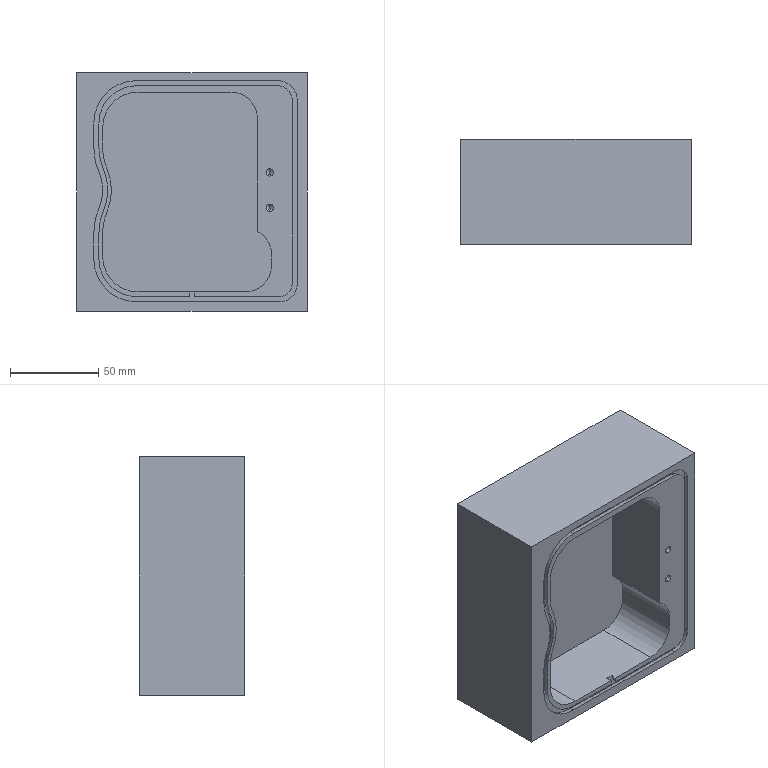Part | STEP file | OP10-144_upper seal block | 1 solid | 82 faces | box 130 x 59.5 x 135 mm | volume 671635 mm3 | cone 30 | plane 28 | cylinder 24 | commonest cylinder face diameters 5 x12 4.2 x4 30 x3 40 x2 60 x2 63 x1